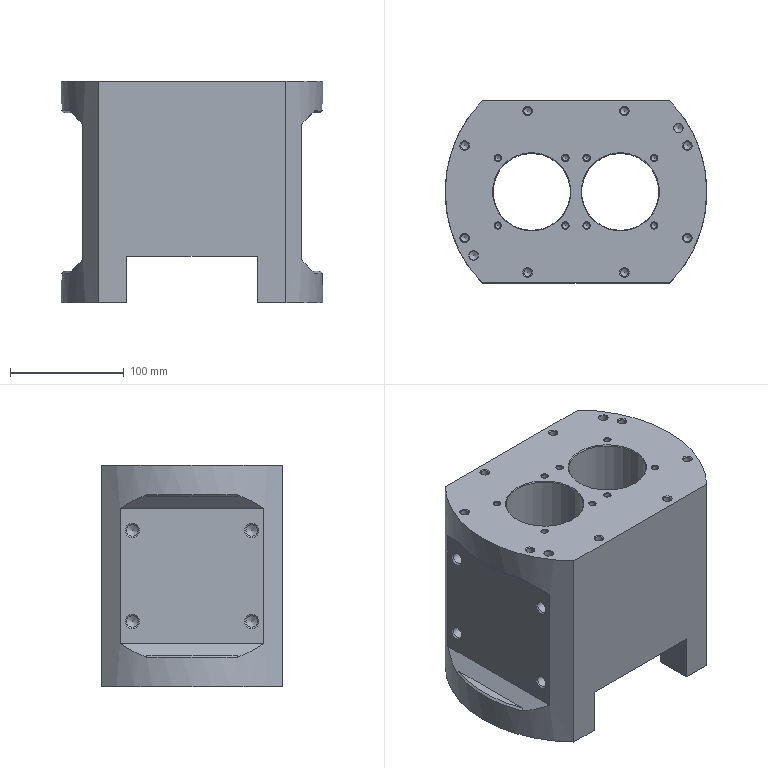NC program | NX | posted with a generic post | part box 230 x 160 x 195 mm
Lines 674 to 1589 of 6533:
(ZLEVEL_PROFILE_COPY_COPY , TOOL : D10)
N1340 T10 M6
N1342 G54
N1344 G17 G0 G90 X68.916 Y-34.13 B0. C0. S3500 M3
N1346 G43 Z30. H10
N1348 Z2.859
N1350 G94 G1 Z-0.141 F1000.
N1352 X70. Y-33.056
N1354 G3 X70.263 Y-32.091 R1.
N1356 G2 X66.402 Y-9.586 R131.143 F2200.
N1358 X67.967 Y21.624 R121.14
N1360 G1 X68.047 Y22.07
N1362 G2 X70.264 Y32.09 R137.442
N1364 G1 X70.265 Y32.27 Z-0.189
N1366 X70.267 Y32.449 Z-0.236
N1368 X70.269 Y32.629 Z-0.283
N1370 G3 X67.196 Y17.784 R137.216
N1372 X66.545 Y-12.585 R119.503
N1374 X70.269 Y-32.628 R131.375
N1376 G1 X70.27 Y-32.807 Z-0.33
N1378 X70.272 Y-32.987 Z-0.377
N1380 X70.274 Y-33.166 Z-0.424
N1382 G2 X66.233 Y-10.924 R132.552
N1384 X67.767 Y22.07 R121.083
N1386 G1 X67.912 Y22.838
N1388 G2 X70.274 Y33.167 R138.495
N1390 G1 Y33.343 Z-0.471
N1392 X70.276 Y33.518 Z-0.519
N1394 X70.28 Y33.692 Z-0.566
N1396 G3 X67.966 Y23.854 R140.229
N1398 G1 X67.879 Y23.408
N1400 G3 X66.093 Y-10.924 R121.238
N1402 X70.28 Y-33.692 R132.326
N1404 G1 X70.281 Y-33.863 Z-0.613
N1406 X70.283 Y-34.033 Z-0.66
N1408 X70.286 Y-34.204 Z-0.707
N1410 G2 X66.081 Y-12.261 R133.
N1412 X67.739 Y23.408 R121.1
N1414 G1 X67.827 Y23.854
N1416 G2 X70.286 Y34.203 R139.429
N1418 G1 Y34.373 Z-0.754
N1420 X70.287 Y34.542 Z-0.801
N1422 X70.292 Y34.711 Z-0.849
N1424 G3 X67.033 Y20.308 R139.647
N1426 X66.48 Y-16.676 R120.009
N1428 X70.291 Y-34.713 R134.78
N1430 G1 X70.29 Y-34.879 Z-0.896
N1432 X70.292 Y-35.044 Z-0.943
N1434 X70.298 Y-35.208 Z-0.99
N1436 G2 X65.996 Y-14.045 R134.124
N1438 X67.46 Y23.408 R120.852
N1440 G1 X67.548 Y23.854
N1442 G2 X70.298 Y35.207 R139.692
N1444 G1 X70.297 Y35.371 Z-1.037
N1446 X70.298 Y35.534 Z-1.084
N1448 X70.303 Y35.696 Z-1.131
N1450 G3 X67.408 Y23.854 R139.78
N1452 G1 X67.32 Y23.408
N1454 G3 X65.856 Y-14.045 R120.758
N1456 X70.303 Y-35.696 R133.625
N1458 G1 X70.302 Y-35.859 Z-1.179
N1460 X70.304 Y-36.022 Z-1.226
N1462 X70.309 Y-36.183 Z-1.273
N1464 G2 X65.879 Y-15.382 R135.159
N1466 X67.18 Y23.408 R120.784
N1468 G1 X67.269 Y23.854
N1470 G2 X70.309 Y36.184 R140.85
N1472 G1 X70.306 Y36.346 Z-1.32
N1474 X70.308 Y36.506 Z-1.367
N1476 X70.314 Y36.665 Z-1.414
N1478 G3 X67.129 Y23.854 R142.003
N1480 G1 X67.04 Y23.408
N1482 G3 X65.982 Y-17.166 R120.703
N1484 X70.314 Y-36.664 R136.659
N1486 G1 X70.313 Y-36.823 Z-1.461
N1488 X70.315 Y-36.98 Z-1.509
N1490 X70.32 Y-37.136 Z-1.556
N1492 G2 X65.78 Y-16.72 R136.306
N1494 X66.989 Y23.854 R120.54
N1496 X70.32 Y37.136 R142.488
N1498 G1 X70.319 Y37.293 Z-1.603
N1500 X70.321 Y37.449 Z-1.65
N1502 X70.325 Y37.604 Z-1.697
N1504 G3 X66.507 Y22.07 R141.233
N1506 X65.704 Y-17.166 R120.238
N1508 X70.325 Y-37.605 R136.58
N1510 G1 X70.324 Y-37.759 Z-1.744
N1512 X70.326 Y-37.913 Z-1.791
N1514 X70.331 Y-38.066 Z-1.839
N1516 G2 X65.977 Y-19.841 R139.717
N1518 X64.478 Y-6.097 R123.724
N1520 X64.4 Y-3.138 R56.152
N1522 G1 Y2.949
N1524 G2 X64.5 Y6.465 R65.963
N1526 G1 X64.643 Y8.694
N1528 X64.673 Y9.14
N1530 G2 X68.111 Y30.096 R126.703
N1532 G1 X68.336 Y30.987
N1534 G2 X70.331 Y38.065 R144.409
N1536 G1 Y38.218 Z-1.886
N1538 X70.334 Y38.37 Z-1.933
N1540 X70.337 Y38.521 Z-1.98
N1542 G3 X68.501 Y32.146 R138.167
N1544 X64.532 Y9.14 R127.538
N1546 X64.4 Y6.386 R43.512
N1548 G1 Y-6.39
N1550 G3 X64.532 Y-9.14 R44.875
N1552 X65.621 Y-18.503 R127.087
N1554 X70.338 Y-38.521 R138.526
N1556 G1 X70.339 Y-38.672 Z-2.028
N1558 X70.341 Y-38.824 Z-2.075
N1560 X70.345 Y-38.975 Z-2.122
N1562 G2 X65.699 Y-19.841 R139.476
N1564 X64.433 Y-9.586 R115.492
N1566 G1 X64.4 Y-8.534
N1568 Y8.539
N1570 G2 X64.47 Y10.032 R16.69
N1572 G1 X64.523 Y10.62
N1574 G2 X68.211 Y31.57 R126.18
N1576 G1 X68.399 Y32.279
N1578 G2 X70.344 Y38.977 R145.55
N1580 G1 X70.345 Y39.129 Z-2.17
N1582 X70.347 Y39.281 Z-2.217
N1584 X70.35 Y39.433 Z-2.264
N1586 G3 X68.022 Y31.38 R158.321
N1588 X64.521 Y12.165 R130.734
N1590 X64.4 Y10.2 R22.35
N1592 G1 Y-10.202
N1594 G3 X64.483 Y-11.744 R18.294
N1596 X65.709 Y-20.733 R114.592
N1598 X70.351 Y-39.429 R141.3
N1600 G1 X70.352 Y-39.58 Z-2.312
N1602 X70.355 Y-39.731 Z-2.359
N1604 X70.359 Y-39.881 Z-2.406
N1606 G2 X65.893 Y-22.516 R143.617
N1608 X64.445 Y-12.707 R115.949
N1610 X64.4 Y-11.708 R15.85
N1612 G1 Y11.703
N1614 G2 X64.476 Y13.006 R12.516
N1616 X67.986 Y31.774 R128.575
N1618 X70.357 Y39.886 R167.552
N1620 G1 X70.359 Y40.037 Z-2.454
N1622 X70.362 Y40.188 Z-2.501
N1624 X70.365 Y40.339 Z-2.549
N1626 X70.274 Y40.051
N1628 X69.128 Y36.338
N1630 G3 X64.614 Y15.382 R133.627
N1632 G1 X64.559 Y14.936
N1634 X64.472 Y14.18
N1636 G3 X64.4 Y13.002 R12.593
N1638 G1 Y-12.999
N1640 G3 X64.487 Y-14.333 R12.788
N1642 X65.923 Y-23.408 R115.066
N1644 X70.367 Y-40.332 R146.297
N1646 G1 X70.369 Y-40.482 Z-2.596
N1648 X70.372 Y-40.633 Z-2.644
N1650 X70.375 Y-40.783 Z-2.691
N1652 G2 X66.286 Y-25.847 R152.499
N1654 X64.514 Y-15.675 R117.501
N1656 G1 X64.49 Y-15.499
N1658 G2 X64.4 Y-14.179 R9.736
N1660 G1 Y14.181
N1662 G2 X64.474 Y15.382 R10.377
N1664 X68.474 Y34.554 R131.136
N1666 X70.372 Y40.791 R204.822
N1668 G1 X70.376 Y40.947 Z-2.739
N1670 X70.379 Y41.104 Z-2.787
N1672 X70.383 Y41.26 Z-2.834
N1674 G3 X68.337 Y34.554 R238.774
N1676 X64.514 Y16.669 R129.735
N1678 X64.4 Y15.265 R9.803
N1680 G1 Y-15.266
N1682 G3 X64.492 Y-16.522 R9.804
N1684 X67.556 Y-31.709 R126.199
N1686 X70.385 Y-41.25 R179.537
N1688 G1 X70.386 Y-41.473 Z-2.906
N1690 X70.388 Y-41.696 Z-2.977
N1692 G2 X68.501 Y-35.597 R288.12
N1694 X64.569 Y-18.057 R132.581
N1696 G1 X64.507 Y-17.611
N1698 G2 X64.4 Y-16.274 R9.898
N1700 G1 Y16.274
N1702 G2 X64.514 Y17.665 R10.021
N1704 G1 X64.569 Y18.057
N1706 G2 X68.987 Y37.229 R135.106
N1708 G1 X70.382 Y41.702
N1710 X70.254 Y41.849 Z-3.12
N1712 G2 X70.151 Y41.386 R2.803
N1714 G1 X68.851 Y37.229
N1716 G3 X64.514 Y18.607 R134.719
N1718 X64.4 Y17.234 R8.61
N1720 G1 Y-17.238
N1722 G3 X64.5 Y-18.522 R8.604
N1724 X65.822 Y-25.637 R117.468
N1726 X69.882 Y-40.512 R148.563
N1728 G2 X70.248 Y-41.817 R14.95
N1730 G1 X70.149 Y-41.701 Z-3.192
N1732 X70.034 Y-41.587 Z-3.264
N1734 G3 X69.897 Y-40.987 R3.303
N1736 G2 X66.286 Y-28.312 R159.77
N1738 X64.505 Y-19.395 R116.11
N1740 X64.4 Y-18.143 R8.464
N1742 G1 Y18.14
N1744 G2 X64.514 Y19.45 R8.464
N1746 X68.714 Y37.229 R133.661
N1748 G1 X70.026 Y41.416
N1750 X70.055 Y41.504
N1752 X70.048 Y41.596
N1754 X70.068 Y41.868
N1756 X70.096 Y42.09
N1758 X70.019 Y42.233 Z-3.335
N1760 X69.945 Y42.375 Z-3.407
N1762 X69.901 Y41.465
N1764 X69.837 Y41.242
N1766 X68.994 Y38.567
N1768 X68.715 Y37.675
N1770 G3 X64.662 Y21.178 R136.319
N1772 G1 X64.514 Y20.293
N1774 G3 X64.4 Y19.003 R8.521
N1776 G1 Y-19.005
N1778 G3 X64.514 Y-20.293 R8.525
N1780 G1 X64.662 Y-21.178
N1782 G3 X67.774 Y-34.511 R131.572
N1784 X69.836 Y-41.242 R222.898
N1786 G2 X69.942 Y-42.377 R9.107
N1788 G1 X69.865 Y-42.518 Z-3.479
N1790 X69.797 Y-42.658 Z-3.551
N1792 G2 X69.758 Y-41.465 R12.32
N1794 G1 X69.7 Y-41.242
N1796 X68.578 Y-37.675
N1798 G2 X64.521 Y-21.178 R135.988
N1800 X64.4 Y-19.828 R8.43
N1802 G1 Y19.826
N1804 G2 X64.535 Y21.256 R8.433
N1806 X68.486 Y37.375 R135.387
N1808 G1 X68.996 Y39.013
N1810 X69.703 Y41.242
N1812 X69.761 Y41.465
N1814 G2 X69.8 Y42.655 R12.703
N1816 G1 X69.721 Y42.793 Z-3.622
N1818 X69.655 Y42.931 Z-3.694
N1820 G3 X69.619 Y41.465 R26.775
N1822 G1 X69.569 Y41.242
N1824 X68.53 Y37.959
N1826 G3 X64.527 Y21.964 R135.005
N1828 X64.4 Y20.616 R7.545
N1830 G1 Y-20.616
N1832 G3 X64.528 Y-21.966 R7.544
N1834 X68.552 Y-38.039 R136.121
N1836 G1 X69.565 Y-41.242
N1838 X69.616 Y-41.465
N1840 G3 X69.65 Y-42.936 R26.513
N1842 G1 X69.57 Y-43.07 Z-3.765
N1844 X69.508 Y-43.204 Z-3.836
N1846 X69.496 Y-43.026
N1848 X69.474 Y-41.465
N1850 X69.43 Y-41.242
N1852 X68.222 Y-37.391
N1854 G2 X65.201 Y-25.997 R131.794
N1856 X64.514 Y-22.614 R121.596
N1858 X64.4 Y-21.371 R7.602
N1860 G1 Y21.374
N1862 G2 X64.535 Y22.731 R7.604
N1864 X68.194 Y37.314 R132.778
N1866 G1 X68.725 Y39.013
N1868 X69.435 Y41.242
N1870 X69.477 Y41.465
N1872 X69.502 Y43.026
N1874 X69.513 Y43.198
N1876 X69.433 Y43.331 Z-3.908
N1878 X69.363 Y43.463 Z-3.979
N1880 X69.336 Y41.465
N1882 X69.301 Y41.242
N1884 X68.248 Y37.919
N1886 G3 X64.539 Y23.483 R134.775
N1888 X64.4 Y22.073 R7.236
N1890 G1 Y-22.072
N1892 G3 X64.535 Y-23.457 R7.198
N1894 X66.856 Y-33.219 R125.973
N1896 X69.264 Y-41.132 R187.049
N1898 G2 X69.333 Y-41.545 R1.376
N1900 G1 X69.356 Y-43.469
N1902 X69.286 Y-43.61 Z-4.05
N1904 X69.224 Y-43.752 Z-4.121
N1906 X69.215 Y-43.471
N1908 X69.191 Y-41.517
N1910 G3 X69.124 Y-41.111 R1.343
N1912 G2 X66.286 Y-31.63 R174.297
N1914 X64.539 Y-24.183 R135.627
N1916 X64.4 Y-22.808 R6.847
N1918 G1 Y22.812
N1920 G2 X64.539 Y24.18 R6.814
N1922 X68.058 Y37.752 R136.135
N1924 G1 X69.167 Y41.242
N1926 X69.195 Y41.465
N1928 X69.222 Y43.471
N1930 X69.231 Y43.744
N1932 X69.156 Y43.9 Z-4.192
N1934 X69.09 Y44.056 Z-4.262
N1936 X69.086 Y43.917
N1938 X69.055 Y41.465
N1940 X69.033 Y41.242
N1942 X68.179 Y38.567
N1944 G3 X64.54 Y24.84 R136.279
N1946 X64.4 Y23.489 R6.572
N1948 G1 Y-23.484
N1950 G3 X64.514 Y-24.714 R7.182
N1952 X66.431 Y-32.675 R120.957
N1954 X68.998 Y-41.138 R181.849
N1956 G2 X69.05 Y-41.447 R1.024
N1958 G1 X69.078 Y-43.917
N1960 X69.083 Y-44.065
N1962 X69.011 Y-44.244 Z-4.333
N1964 X68.943 Y-44.422 Z-4.404
N1966 X68.938 Y-43.917
N1968 X68.909 Y-41.465
N1970 X68.893 Y-41.242
N1972 G2 X66.932 Y-34.921 R233.838
N1974 X64.537 Y-25.454 R125.397
N1976 X64.4 Y-24.148 R6.303
N1978 G1 Y24.143
N1980 G2 X64.539 Y25.465 R6.339
N1982 X67.828 Y37.874 R131.335
N1984 G1 X68.899 Y41.242
N1986 X68.915 Y41.465
N1988 X68.945 Y43.917
N1990 X68.949 Y44.415
N1992 X68.878 Y44.594 Z-4.475
N1994 X68.809 Y44.774 Z-4.545
N1996 X68.775 Y41.465
N1998 X68.763 Y41.242
N2000 X68.624 Y40.796
N2002 X67.87 Y38.447
N2004 G3 X64.568 Y26.248 R136.583
N2006 X64.4 Y24.745 R7.116
N2008 G1 Y-24.765
N2010 G3 X64.546 Y-26.124 R6.411
N2012 X66.776 Y-34.855 R123.118
N2014 X68.757 Y-41.242 R239.84
N2016 G1 X68.769 Y-41.465
N2018 X68.805 Y-44.779
N2020 X68.735 Y-44.956 Z-4.616
N2022 X68.669 Y-45.133 Z-4.687
N2024 X68.628 Y-41.465
N2026 X68.621 Y-41.242
N2028 X67.213 Y-36.784
N2030 X66.943 Y-35.892
N2032 G2 X64.553 Y-26.784 R133.26
N2034 X64.4 Y-25.405 R6.284
N2036 G1 Y25.4
N2038 G2 X64.593 Y26.975 R6.887
N2040 X67.916 Y39.013 R138.537
N2042 G1 X68.501 Y40.829
N2044 X68.628 Y41.242
N2046 X68.671 Y45.13
N2048 X68.598 Y45.306 Z-4.757
N2050 X68.532 Y45.482 Z-4.828
N2052 X68.492 Y41.242
N2054 X68.429 Y41.019
N2056 X67.782 Y39.013
N2058 G3 X64.553 Y27.399 R138.721
N2060 X64.4 Y26.058 R5.941
N2062 G1 Y-26.052
N2064 G3 X64.554 Y-27.402 R5.992
N2066 X67.379 Y-37.743 R135.651
N2068 G1 X68.485 Y-41.242
N2070 X68.53 Y-45.484
N2072 X68.456 Y-45.658 Z-4.899
N2074 X68.39 Y-45.832 Z-4.97
N2076 X68.345 Y-41.242
N2078 X68.217 Y-40.796
N2080 X67.502 Y-38.567
N2082 G2 X64.559 Y-27.984 R134.533
N2084 X64.4 Y-26.609 R6.02
N2086 G1 Y26.602
N2088 G2 X64.587 Y28.137 R6.891
N2090 X67.538 Y38.672 R138.816
N2092 G1 X68.296 Y41.019
N2094 X68.352 Y41.242
N2096 X68.392 Y45.83
N2098 X68.317 Y46.004 Z-5.04
N2100 X68.248 Y46.179 Z-5.111
N2102 X68.222 Y42.134
N2104 X68.212 Y41.242
N2106 G2 X68.139 Y40.938 R2.011
N2108 G1 X67.95 Y40.35
N2110 G3 X64.565 Y28.574 R137.526
N2112 X64.4 Y27.181 R5.974
N2114 G1 Y-27.182
N2116 G3 X64.563 Y-28.567 R5.956
N2118 X67.509 Y-39.013 R135.107
N2120 G1 X68.083 Y-40.796
N2122 X68.206 Y-41.242
N2124 G2 X68.247 Y-46.18 R273.815
N2126 G1 X68.175 Y-46.354 Z-5.182
N2128 X68.107 Y-46.528 Z-5.252
N2130 G3 X68.067 Y-41.242 R301.682
N2132 X67.702 Y-40.021 R20.81
N2134 G2 X64.578 Y-29.21 R143.238
N2136 X64.4 Y-27.749 R6.092
N2138 G1 Y27.748
N2140 G2 X64.583 Y29.238 R6.142
N2142 X68.058 Y41.104 R155.223
N2144 G1 X68.072 Y41.242
N2146 X68.108 Y46.527
N2148 X68.035 Y46.697 Z-5.323
N2150 X67.968 Y46.866 Z-5.394
N2152 X67.942 Y42.134
N2154 X67.932 Y41.242
N2156 G2 X67.798 Y40.691 R3.274
N2158 G3 X64.586 Y29.803 R142.667
N2160 X64.4 Y28.302 R6.139
N2162 G1 Y-28.302
N2164 G3 X64.587 Y-29.806 R6.142
N2166 X67.587 Y-40.078 R145.418
N2168 G2 X67.929 Y-41.242 R17.07
N2170 G1 X67.941 Y-42.134
N2172 X67.967 Y-46.867
N2174 X67.893 Y-47.035 Z-5.465
N2176 X67.826 Y-47.203 Z-5.535
N2178 X67.802 Y-42.134
N2180 X67.791 Y-41.242
N2182 G3 X67.457 Y-40.091 R15.159
N2184 G2 X64.587 Y-30.329 R143.266
N2186 X64.4 Y-28.844 R5.995
N2188 G1 Y28.844
N2190 G2 X64.587 Y30.329 R5.995
N2192 X67.733 Y40.903 R142.222
N2194 G3 X67.793 Y41.26 R1.127
N2196 G1 X67.823 Y46.592
N2198 X67.827 Y47.203
N2200 X67.752 Y47.371 Z-5.606
N2202 X67.684 Y47.54 Z-5.677
N2204 X67.671 Y43.026
N2206 X67.653 Y41.244
N2208 G2 X67.635 Y41.019 R1.6
N2210 G3 X64.627 Y31.048 R153.55
N2212 X64.4 Y29.374 R6.83
N2214 G1 Y-29.371
N2216 G3 X64.514 Y-30.543 R6.829
N2218 X67.326 Y-40.099 R135.473
N2220 G2 X67.653 Y-41.242 R13.322
N2222 G1 X67.663 Y-42.134
N2224 X67.684 Y-47.54
N2226 X67.611 Y-47.708 Z-5.747
N2228 X67.541 Y-47.876 Z-5.818
N2230 X67.524 Y-42.134
N2232 X67.515 Y-41.242
N2234 G3 X67.429 Y-40.85 R2.16
N2236 G1 X66.342 Y-37.448
N2238 G2 X64.575 Y-31.29 R107.735
N2240 X64.4 Y-29.897 R5.633
N2242 G1 Y29.93
N2244 G2 X64.571 Y31.272 R5.342
N2246 X67.5 Y41.019 R134.235
N2248 G3 X67.541 Y47.876 R318.564
N2250 G1 X67.47 Y48.041 Z-5.889
N2252 X67.405 Y48.205 Z-5.96
N2254 X67.383 Y42.134
N2256 X67.366 Y41.019
N2258 G3 X64.602 Y31.932 R148.181
N2260 X64.4 Y30.41 R5.852
N2262 G1 Y-30.409
N2264 G3 X64.602 Y-31.935 R5.857
N2266 X67.229 Y-40.628 R151.989
N2268 G2 X67.378 Y-41.242 R3.709
N2270 G1 X67.405 Y-48.205
N2272 X67.328 Y-48.369 Z-6.03
N2274 X67.262 Y-48.532 Z-6.101
N2276 X67.245 Y-41.386
N2278 G3 X67.14 Y-40.754 R1.995
N2280 G2 X64.611 Y-32.473 R152.322
N2282 X64.4 Y-30.912 R5.895
N2284 G1 Y30.91
N2286 G2 X64.616 Y32.496 R5.93
N2288 X67.231 Y41.019 R165.339
N2290 G1 X67.244 Y42.134
N2292 X67.262 Y48.532
N2294 X67.187 Y48.694 Z-6.172
N2296 X67.118 Y48.856 Z-6.242
N2298 X67.106 Y42.58
N2300 X67.094 Y41.019
N2302 X67.032 Y40.796
N2304 X66.97 Y40.614
N2306 G3 X64.648 Y33.126 R149.7
N2308 X64.4 Y31.402 R6.641
N2310 G1 Y-31.404
N2312 G3 X64.674 Y-33.217 R6.643
N2314 X67.093 Y-41.019 R175.153
N2316 G1 X67.103 Y-41.242
N2318 X67.118 Y-48.856
N2320 X67.045 Y-49.019 Z-6.313
N2322 X66.978 Y-49.181 Z-6.384
N2324 X66.965 Y-41.242
N2326 X66.959 Y-41.019
N2328 G2 X64.669 Y-33.662 R172.96
N2330 X64.4 Y-31.887 R6.178
N2332 G1 Y31.892
N2334 G2 X64.623 Y33.498 R5.902
N2336 X66.898 Y40.796 R143.482
N2338 G1 X66.954 Y41.019
N2340 X66.964 Y42.134
N2342 X66.978 Y49.181
N2344 X66.904 Y49.341 Z-6.455
N2346 X66.838 Y49.502 Z-6.525
N2348 X66.825 Y42.134
N2350 X66.815 Y41.019
N2352 X66.765 Y40.796
N2354 G3 X64.665 Y34.108 R137.782
N2356 X64.4 Y32.365 R6.15
N2358 G1 Y-32.366
N2360 G3 X64.665 Y-34.108 R6.15
N2362 G1 X65.321 Y-36.338
N2364 G3 X66.824 Y-41.019 R284.979
N2366 G1 X66.827 Y-41.242
N2368 X66.833 Y-49.268
N2370 X66.838 Y-49.502
N2372 X66.763 Y-49.661 Z-6.596
N2374 X66.695 Y-49.819 Z-6.667
N2376 X66.688 Y-41.019
N2378 X66.627 Y-40.796
N2380 X66.329 Y-39.905
N2382 G2 X64.661 Y-34.554 R130.92
N2384 X64.4 Y-32.835 R6.126
N2386 G1 Y32.836
N2388 G2 X64.661 Y34.554 R6.127
N2390 X66.631 Y40.796 R132.059
N2392 G1 X66.643 Y40.839
N2394 X66.676 Y41.019
N2396 X66.682 Y41.688
N2398 X66.695 Y49.819
N2400 X66.621 Y49.976 Z-6.737
N2402 X66.551 Y50.133 Z-6.808
N2404 X66.543 Y41.688
N2406 X66.537 Y41.058
N2408 G2 X66.486 Y40.762 R0.94
N2410 G3 X64.657 Y35. R132.97
N2412 X64.4 Y33.298 R6.101
N2414 G1 Y-33.298
N2416 G3 X64.657 Y-35. R6.101
N2418 G1 X64.917 Y-35.892
N2420 X66.046 Y-39.459
N2422 X66.286 Y-40.171
N2424 X66.517 Y-40.875
N2426 X66.547 Y-41.019
N2428 X66.551 Y-50.133
N2430 X66.48 Y-50.29 Z-6.879
N2432 X66.413 Y-50.446 Z-6.949
N2434 X66.409 Y-50.159
N2436 X66.407 Y-42.58
N2438 Y-41.019
N2440 X66.364 Y-40.796
N2442 G2 X64.653 Y-35.446 R141.656
N2444 X64.4 Y-33.754 R6.117
N2446 G1 Y33.755
N2448 G2 X64.653 Y35.446 R6.118
N2450 X66.356 Y40.772 R138.84
N2452 G3 X66.397 Y41.011 R0.761
N2454 G1 X66.403 Y41.688
N2456 X66.409 Y50.159
N2458 X66.413 Y50.446
N2460 X66.338 Y50.603 Z-7.02
N2462 X66.271 Y50.759 Z-7.091
N2464 X66.26 Y40.95
N2466 X66.25 Y40.853
N2468 G3 X64.648 Y35.892 R152.438
N2470 X64.4 Y34.203 R6.104
N2472 G1 Y-34.203
N2474 G3 X64.648 Y-35.892 R6.105
N2476 X66.254 Y-40.864 R148.591
N2478 G1 X66.266 Y-40.977
N2480 X66.271 Y-50.759
N2482 X66.197 Y-50.914 Z-7.162
N2484 X66.127 Y-51.069 Z-7.232
N2486 X66.125 Y-40.941
N2488 X66.116 Y-40.856
N2490 G2 X64.651 Y-36.338 R159.842
N2492 X64.4 Y-34.647 R5.955
N2494 G1 Y34.648
N2496 G2 X64.651 Y36.338 R5.956
N2498 X66.114 Y40.85 R164.319
N2500 G1 X66.121 Y40.925
N2502 X66.127 Y51.069
N2504 X66.056 Y51.22 Z-7.303
N2506 X65.988 Y51.372 Z-7.374
N2508 X65.985 Y51.051
N2510 X65.983 Y40.902
N2512 X65.977 Y40.844
N2514 G3 X64.659 Y36.784 R153.678
N2516 X64.4 Y35.082 R5.892
N2518 G1 Y-35.082
N2520 G3 X64.659 Y-36.784 R5.892
N2522 X65.979 Y-40.848 R159.856
N2524 G1 X65.985 Y-40.906
N2526 Y-51.051
N2528 X65.988 Y-51.372
N2530 X65.914 Y-51.523 Z-7.444
N2532 X65.846 Y-51.675 Z-7.515
N2534 X65.843 Y-51.497
N2536 Y-41.074
N2538 Y-40.826
N2540 G2 X64.667 Y-37.229 R116.234
N2542 X64.4 Y-35.514 R5.916
N2544 G1 Y35.515
N2546 G2 X64.667 Y37.229 R5.916
N2548 X65.843 Y40.826 R116.234
N2550 G1 Y41.074
N2552 X65.841 Y42.134
N2554 X65.843 Y51.497
N2556 X65.846 Y51.675
N2558 X65.773 Y51.826 Z-7.586
N2560 X65.704 Y51.977 Z-7.657
N2562 X65.702 Y51.943
N2564 X65.701 Y41.688
N2566 X65.702 Y41.443
N2568 Y40.809
N2570 G3 X64.674 Y37.675 R116.063
N2572 X64.4 Y35.938 R5.941
N2574 G1 Y-35.938
N2576 G3 X64.674 Y-37.675 R5.941
N2578 X65.702 Y-40.809 R115.984
N2580 G1 Y-41.444
N2582 Y-51.943
N2584 X65.704 Y-51.977
N2586 X65.631 Y-52.129 Z-7.727
N2588 X65.566 Y-52.28 Z-7.798
N2590 X65.561 Y-51.943
N2592 Y-41.807
N2594 Y-40.783
N2596 X64.822 Y-38.567
N2598 X64.682 Y-38.121
N2600 G2 X64.4 Y-36.338 R5.959
N2602 G1 Y36.338
N2604 G2 X64.682 Y38.121 R5.959
N2606 G1 X64.822 Y38.567
N2608 X65.561 Y40.783
N2610 Y41.807
N2612 X65.559 Y42.134
N2614 X65.561 Y51.943
N2616 X65.566 Y52.28
N2618 X65.49 Y52.428 Z-7.869
N2620 X65.423 Y52.576 Z-7.939
N2622 X65.419 Y52.389
N2624 Y42.134
N2626 Y40.757
N2628 X64.69 Y38.567
N2630 G3 X64.4 Y36.771 R5.975
N2632 G1 Y-36.772
N2634 G3 X64.69 Y-38.567 R5.975
N2636 G1 X65.419 Y-40.757
N2638 Y-42.134
N2640 Y-52.389
N2642 X65.423 Y-52.576
N2644 X65.348 Y-52.723 Z-8.01
N2646 X65.28 Y-52.869 Z-8.081
N2648 X65.278 Y-52.834
N2650 Y-42.525
N2652 Y-40.796
N2654 X65.277 Y-40.721
N2656 X64.699 Y-39.013
N2658 G2 X64.4 Y-37.182 R5.897
N2660 G1 Y37.183
N2662 G2 X64.699 Y39.013 R5.897
N2664 G1 X65.277 Y40.721
N2666 X65.278 Y40.796
N2668 Y42.525
N2670 Y52.834
N2672 X65.28 Y52.869
N2674 X65.207 Y53.016 Z-8.152
N2676 X65.141 Y53.162 Z-8.222
N2678 X65.136 Y52.834
N2680 X65.135 Y42.879
N2682 X65.136 Y42.58
N2684 Y40.796
N2686 Y40.695
N2688 X64.717 Y39.459
N2690 G3 X64.4 Y37.585 R5.802
N2692 G1 Y-37.585
N2694 G3 X64.717 Y-39.459 R5.802
N2696 G1 X65.136 Y-40.695
N2698 Y-40.796
N2700 Y-42.58
N2702 Y-52.834
N2704 X65.141 Y-53.162
N2706 X65.066 Y-53.309 Z-8.293
N2708 X64.999 Y-53.455 Z-8.364
N2710 X64.995 Y-53.28
N2712 Y-43.026
N2714 Y-40.796
N2716 X64.994 Y-40.669
N2718 G2 X64.629 Y-39.562 R20.679
N2720 X64.4 Y-37.997 R5.463
N2722 G1 Y37.997
N2724 G2 X64.629 Y39.562 R5.463
N2726 X64.994 Y40.669 R20.679
N2728 G1 X64.995 Y40.796
N2730 Y43.229
N2732 Y53.28
N2734 X64.999 Y53.455
N2736 X64.924 Y53.601 Z-8.434
N2738 X64.855 Y53.747 Z-8.505
N2740 X64.852 Y43.577
N2742 X64.853 Y43.471
N2744 Y40.643
N2746 X64.698 Y40.187
N2748 G3 X64.4 Y38.381 R5.618
N2750 G1 Y-38.381
N2752 G3 X64.698 Y-40.187 R5.618
N2754 G1 X64.853 Y-40.643
N2756 Y-43.471
N2758 X64.855 Y-53.747
N2760 X64.783 Y-53.89 Z-8.576
N2762 X64.717 Y-54.032 Z-8.647
N2764 X64.712 Y-53.726
N2766 Y-43.921
N2768 Y-40.611
N2770 G2 X64.4 Y-38.77 R5.654
N2772 G1 Y38.77
N2774 G2 X64.712 Y40.611 R5.653
N2776 G1 Y43.92
N2778 X64.711 Y44.363
N2780 X64.712 Y53.726
N2782 X64.717 Y54.032
N2784 X64.641 Y54.174 Z-8.717
N2786 X64.574 Y54.316 Z-8.788
N2788 X64.571 Y54.172
N2790 Y43.917
N2792 Y40.541
N2794 G3 X64.4 Y39.155 R6.379
N2796 G1 Y-39.155
N2798 G3 X64.571 Y-40.541 R6.38
N2800 G1 Y-43.917
N2802 Y-54.172
N2804 X64.574 Y-54.316
N2806 X64.5 Y-54.458 Z-8.859
N2808 X64.43 Y-54.6 Z-8.929
N2810 X64.429 Y-44.363
N2812 Y-40.16
N2814 X64.4 Y-39.536
N2816 Y39.536
N2818 X64.429 Y40.16
N2820 Y44.599
N2822 X64.43 Y54.6
N2824 X64.358 Y54.741 Z-9.
N2826 X64.294 Y54.883 Z-9.071
N2828 X64.288 Y54.618
N2830 Y44.809
N2832 Y-44.809
N2834 Y-54.618
N2836 X64.294 Y-54.883
N2838 X64.217 Y-55.024 Z-9.142
N2840 X64.15 Y-55.165 Z-9.212
N2842 X64.146 Y-55.064
N2844 Y-45.267
N2846 Y45.266
N2848 Y55.064
N2850 X64.15 Y55.165
N2852 X64.076 Y55.303 Z-9.283
N2854 X64.006 Y55.442 Z-9.354
N2856 X64.005 Y45.255
N2858 Y-45.255
N2860 X64.004 Y-45.701
N2862 X64.006 Y-55.442
N2864 X63.934 Y-55.579 Z-9.424
N2866 X63.87 Y-55.716 Z-9.495
N2868 X63.864 Y-55.51
N2870 Y-45.922
N2872 Y45.922
N2874 Y55.51
N2876 X63.87 Y55.716
N2878 X63.793 Y55.853 Z-9.566
N2880 X63.724 Y55.99 Z-9.636
N2882 X63.722 Y46.147
N2884 Y-46.147
N2886 X63.724 Y-55.99
N2888 X63.651 Y-56.128 Z-9.707
N2890 X63.583 Y-56.265 Z-9.778
N2892 X63.581 Y-55.956
N2894 Y-46.147
N2896 Y55.956
N2898 X63.583 Y56.265
N2900 X63.51 Y56.401 Z-9.849
N2902 X63.445 Y56.537 Z-9.919
N2904 X63.439 Y56.401
N2906 X63.438 Y46.883
N2908 X63.439 Y46.592
N2910 Y-46.592
N2912 X63.438 Y-46.883
N2914 X63.439 Y-56.401
N2916 X63.445 Y-56.537
N2918 X63.369 Y-56.672 Z-9.99
N2920 X63.3 Y-56.806 Z-10.061
N2922 X63.298 Y-47.038
N2924 Y47.2
N2926 X63.3 Y56.806
N2928 X63.227 Y56.94 Z-10.131
N2930 X63.159 Y57.073 Z-10.202
N2932 X63.156 Y56.847
N2934 Y-56.847
N2936 X63.159 Y-57.073
N2938 X63.086 Y-57.206 Z-10.273
N2940 X63.018 Y-57.339 Z-10.344
N2942 X63.015 Y-57.293
N2944 Y57.293
N2946 X63.018 Y57.339
N2948 X62.944 Y57.472 Z-10.414
N2950 X62.879 Y57.604 Z-10.485
N2952 X62.874 Y57.293
N2954 X62.873 Y48.13
N2956 X62.874 Y47.93
N2958 Y-57.293
N2960 X62.879 Y-57.604
N2962 X62.803 Y-57.737 Z-10.556
N2964 X62.735 Y-57.87 Z-10.626
N2966 X62.732 Y-57.739
N2968 Y57.739
N2970 X62.735 Y57.87
N2972 X62.661 Y58.001 Z-10.697
N2974 X62.592 Y58.131 Z-10.768
N2976 X62.591 Y48.376
N2978 Y-48.376
N2980 X62.592 Y-58.131
N2982 X62.52 Y-58.26 Z-10.839
N2984 X62.453 Y-58.389 Z-10.909
N2986 X62.449 Y-58.185
N2988 Y58.185
N2990 X62.453 Y58.389
N2992 X62.379 Y58.518 Z-10.98
N2994 X62.309 Y58.647 Z-11.051
N2996 X62.308 Y49.268
N2998 Y-49.268
N3000 X62.309 Y-58.647
N3002 X62.237 Y-58.776 Z-11.121
N3004 X62.17 Y-58.905 Z-11.192
N3006 X62.166 Y-58.631
N3008 Y58.631
N3010 X62.17 Y58.905
N3012 X62.096 Y59.033 Z-11.263
N3014 X62.028 Y59.162 Z-11.334
N3016 X62.025 Y59.077
N3018 Y-59.077
N3020 X62.028 Y-59.162
N3022 X61.954 Y-59.289 Z-11.404
N3024 X61.886 Y-59.417 Z-11.475
N3026 X61.884 Y-50.159
N3028 Y50.159
N3030 X61.886 Y59.417
N3032 X61.813 Y59.543 Z-11.546
N3034 X61.747 Y59.668 Z-11.616
N3036 X61.742 Y59.522
N3038 Y-59.522
N3040 X61.747 Y-59.668
N3042 X61.671 Y-59.793 Z-11.687
N3044 X61.603 Y-59.918 Z-11.758
N3046 X61.601 Y-59.522
N3048 Y59.522
N3050 X61.603 Y59.918
N3052 X61.53 Y60.043 Z-11.829
N3054 X61.463 Y60.168 Z-11.899
N3056 X61.459 Y59.968
N3058 Y-59.968
N3060 X61.463 Y-60.168
N3062 X61.389 Y-60.293 Z-11.97
N3064 X61.318 Y-60.418 Z-12.041
N3066 X61.317 Y-51.497
N3068 X61.318 Y-51.051
N3070 Y51.375
N3072 Y60.418
N3074 X61.247 Y60.542 Z-12.111
N3076 X61.182 Y60.666 Z-12.182
N3078 X61.177 Y60.414
N3080 Y-60.414
N3082 X61.182 Y-60.666
N3084 X61.106 Y-60.789 Z-12.253
N3086 X61.038 Y-60.912 Z-12.323
N3088 X61.035 Y-60.86
N3090 Y60.86
N3092 X61.038 Y60.912
N3094 X60.964 Y61.034 Z-12.394
N3096 X60.896 Y61.155 Z-12.465
N3098 X60.894 Y60.86
N3100 Y-60.86
N3102 X60.896 Y-61.155
N3104 X60.823 Y-61.276 Z-12.536
N3106 X60.755 Y-61.397 Z-12.606
N3108 X60.752 Y-61.306
N3110 Y61.306
N3112 X60.755 Y61.397
N3114 X60.682 Y61.518 Z-12.677
N3116 X60.614 Y61.64 Z-12.748
N3118 X60.611 Y61.306
N3120 Y-61.306
N3122 X60.614 Y-61.64
N3124 X60.54 Y-61.761 Z-12.818
N3126 X60.473 Y-61.881 Z-12.889
N3128 X60.469 Y-61.752
N3130 Y61.752
N3132 X60.473 Y61.881
N3134 X60.399 Y62.002 Z-12.96
N3136 X60.33 Y62.122 Z-13.031
N3138 X60.328 Y61.752
N3140 Y-61.752
N3142 X60.33 Y-62.122
N3144 X60.257 Y-62.241 Z-13.101
N3146 X60.19 Y-62.359 Z-13.172
N3148 X60.187 Y-62.198
N3150 Y62.198
N3152 X60.19 Y62.359
N3154 X60.116 Y62.477 Z-13.243
N3156 X60.046 Y62.594 Z-13.313
N3158 X60.045 Y53.726
N3160 Y-53.726
N3162 X60.046 Y-62.594
N3164 X59.974 Y-62.712 Z-13.384